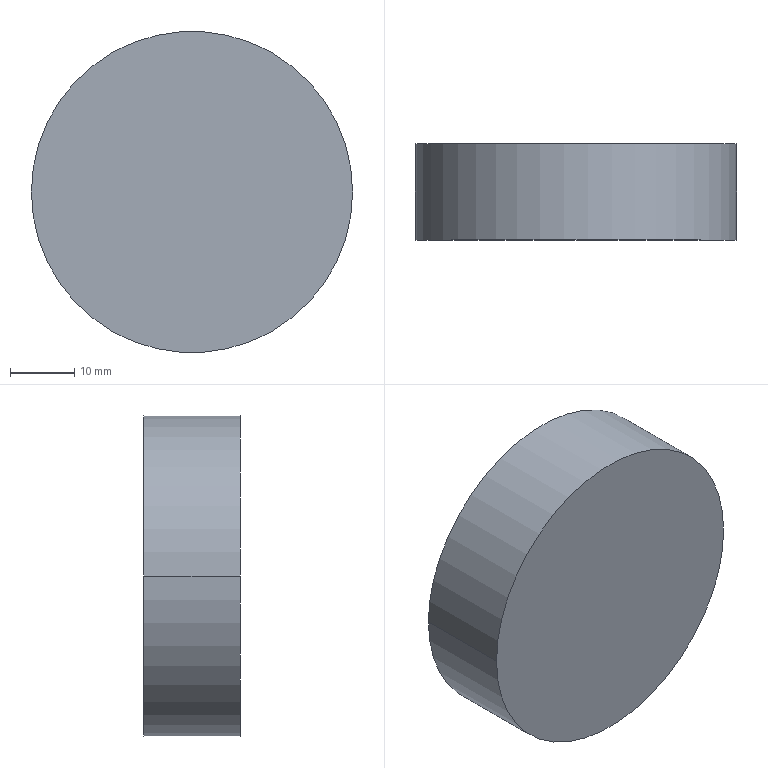Part | NX | 1 solid | 7 faces | box 50 x 15 x 50 mm | volume 11206 mm3 | cylinder 4 | plane 3 | commonest cylinder face diameters 44 x2 50 x2
STEP:
#1=CARTESIAN_POINT('',(-25.,0.,0.));
#2=VERTEX_POINT('',#1);
#3=CARTESIAN_POINT('',(25.,0.,0.));
#4=VERTEX_POINT('',#3);
#5=CARTESIAN_POINT('',(0.,0.,0.));
#6=DIRECTION('',(0.,1.,0.));
#7=DIRECTION('',(1.,0.,0.));
#8=AXIS2_PLACEMENT_3D('',#5,#6,#7);
#9=CIRCLE('',#8,25.);
#10=EDGE_CURVE('',#2,#4,#9,.T.);
#11=ORIENTED_EDGE('',*,*,#10,.F.);
#12=CARTESIAN_POINT('',(0.,0.,0.));
#13=DIRECTION('',(0.,1.,0.));
#14=DIRECTION('',(1.,0.,0.));
#15=AXIS2_PLACEMENT_3D('',#12,#13,#14);
#16=CIRCLE('',#15,25.);
#17=EDGE_CURVE('',#4,#2,#16,.T.);
#18=ORIENTED_EDGE('',*,*,#17,.F.);
#19=EDGE_LOOP('',(#11,#18));
#20=FACE_BOUND('',#19,.T.);
#21=CARTESIAN_POINT('',(0.,0.,0.));
#22=DIRECTION('',(0.,1.,0.));
#23=DIRECTION('',(1.,0.,0.));
#24=AXIS2_PLACEMENT_3D('',#21,#22,#23);
#25=PLANE('',#24);
#26=ADVANCED_FACE('',(#20),#25,.F.);
#27=ORIENTED_EDGE('',*,*,#10,.T.);
#28=CARTESIAN_POINT('',(25.,15.,0.));
#29=VERTEX_POINT('',#28);
#30=CARTESIAN_POINT('',(25.,0.,0.));
#31=DIRECTION('',(0.,1.,0.));
#32=VECTOR('',#31,1000.);
#33=LINE('',#30,#32);
#34=EDGE_CURVE('',#29,#4,#33,.F.);
#35=ORIENTED_EDGE('',*,*,#34,.F.);
#36=CARTESIAN_POINT('',(-25.,15.,0.));
#37=VERTEX_POINT('',#36);
#38=CARTESIAN_POINT('',(0.,15.,0.));
#39=DIRECTION('',(0.,-1.,0.));
#40=DIRECTION('',(-1.,0.,0.));
#41=AXIS2_PLACEMENT_3D('',#38,#39,#40);
#42=CIRCLE('',#41,25.);
#43=EDGE_CURVE('',#29,#37,#42,.T.);
#44=ORIENTED_EDGE('',*,*,#43,.T.);
#45=CARTESIAN_POINT('',(-25.,0.,0.));
#46=DIRECTION('',(0.,1.,0.));
#47=VECTOR('',#46,1000.);
#48=LINE('',#45,#47);
#49=EDGE_CURVE('',#37,#2,#48,.F.);
#50=ORIENTED_EDGE('',*,*,#49,.T.);
#51=EDGE_LOOP('',(#27,#35,#44,#50));
#52=FACE_BOUND('',#51,.T.);
#53=CARTESIAN_POINT('',(0.,0.,0.));
#54=DIRECTION('',(0.,1.,0.));
#55=DIRECTION('',(-1.,0.,0.));
#56=AXIS2_PLACEMENT_3D('',#53,#54,#55);
#57=CYLINDRICAL_SURFACE('',#56,25.);
#58=ADVANCED_FACE('',(#52),#57,.T.);
#59=CARTESIAN_POINT('',(-22.,3.,0.));
#60=VERTEX_POINT('',#59);
#61=CARTESIAN_POINT('',(22.,3.,0.));
#62=VERTEX_POINT('',#61);
#63=CARTESIAN_POINT('',(0.,3.,0.));
#64=DIRECTION('',(0.,-1.,0.));
#65=DIRECTION('',(1.,0.,0.));
#66=AXIS2_PLACEMENT_3D('',#63,#64,#65);
#67=CIRCLE('',#66,22.);
#68=EDGE_CURVE('',#60,#62,#67,.T.);
#69=ORIENTED_EDGE('',*,*,#68,.F.);
#70=CARTESIAN_POINT('',(0.,3.,0.));
#71=DIRECTION('',(0.,-1.,0.));
#72=DIRECTION('',(1.,0.,0.));
#73=AXIS2_PLACEMENT_3D('',#70,#71,#72);
#74=CIRCLE('',#73,22.);
#75=EDGE_CURVE('',#62,#60,#74,.T.);
#76=ORIENTED_EDGE('',*,*,#75,.F.);
#77=EDGE_LOOP('',(#69,#76));
#78=FACE_BOUND('',#77,.T.);
#79=CARTESIAN_POINT('',(0.,3.,0.));
#80=DIRECTION('',(0.,1.,0.));
#81=DIRECTION('',(1.,0.,0.));
#82=AXIS2_PLACEMENT_3D('',#79,#80,#81);
#83=PLANE('',#82);
#84=ADVANCED_FACE('',(#78),#83,.T.);
#85=ORIENTED_EDGE('',*,*,#43,.F.);
#86=CARTESIAN_POINT('',(0.,15.,0.));
#87=DIRECTION('',(0.,-1.,0.));
#88=DIRECTION('',(-1.,0.,0.));
#89=AXIS2_PLACEMENT_3D('',#86,#87,#88);
#90=CIRCLE('',#89,25.);
#91=EDGE_CURVE('',#37,#29,#90,.T.);
#92=ORIENTED_EDGE('',*,*,#91,.F.);
#93=EDGE_LOOP('',(#85,#92));
#94=FACE_BOUND('',#93,.T.);
#95=CARTESIAN_POINT('',(22.,15.,0.));
#96=VERTEX_POINT('',#95);
#97=CARTESIAN_POINT('',(-22.,15.,0.));
#98=VERTEX_POINT('',#97);
#99=CARTESIAN_POINT('',(0.,15.,0.));
#100=DIRECTION('',(0.,1.,0.));
#101=DIRECTION('',(1.,0.,0.));
#102=AXIS2_PLACEMENT_3D('',#99,#100,#101);
#103=CIRCLE('',#102,22.);
#104=EDGE_CURVE('',#96,#98,#103,.T.);
#105=ORIENTED_EDGE('',*,*,#104,.F.);
#106=CARTESIAN_POINT('',(0.,15.,0.));
#107=DIRECTION('',(0.,1.,0.));
#108=DIRECTION('',(1.,0.,0.));
#109=AXIS2_PLACEMENT_3D('',#106,#107,#108);
#110=CIRCLE('',#109,22.);
#111=EDGE_CURVE('',#98,#96,#110,.T.);
#112=ORIENTED_EDGE('',*,*,#111,.F.);
#113=EDGE_LOOP('',(#105,#112));
#114=FACE_BOUND('',#113,.T.);
#115=CARTESIAN_POINT('',(0.,15.,0.));
#116=DIRECTION('',(0.,1.,0.));
#117=DIRECTION('',(1.,0.,0.));
#118=AXIS2_PLACEMENT_3D('',#115,#116,#117);
#119=PLANE('',#118);
#120=ADVANCED_FACE('',(#94,#114),#119,.T.);
#121=ORIENTED_EDGE('',*,*,#104,.T.);
#122=CARTESIAN_POINT('',(-22.,0.,0.));
#123=DIRECTION('',(0.,1.,0.));
#124=VECTOR('',#123,1000.);
#125=LINE('',#122,#124);
#126=EDGE_CURVE('',#98,#60,#125,.F.);
#127=ORIENTED_EDGE('',*,*,#126,.T.);
#128=ORIENTED_EDGE('',*,*,#68,.T.);
#129=CARTESIAN_POINT('',(22.,0.,0.));
#130=DIRECTION('',(0.,1.,0.));
#131=VECTOR('',#130,1000.);
#132=LINE('',#129,#131);
#133=EDGE_CURVE('',#96,#62,#132,.F.);
#134=ORIENTED_EDGE('',*,*,#133,.F.);
#135=EDGE_LOOP('',(#121,#127,#128,#134));
#136=FACE_BOUND('',#135,.T.);
#137=CARTESIAN_POINT('',(0.,0.,0.));
#138=DIRECTION('',(0.,1.,0.));
#139=DIRECTION('',(-1.,0.,0.));
#140=AXIS2_PLACEMENT_3D('',#137,#138,#139);
#141=CYLINDRICAL_SURFACE('',#140,22.);
#142=ADVANCED_FACE('',(#136),#141,.F.);
#143=ORIENTED_EDGE('',*,*,#49,.F.);
#144=ORIENTED_EDGE('',*,*,#91,.T.);
#145=ORIENTED_EDGE('',*,*,#34,.T.);
#146=ORIENTED_EDGE('',*,*,#17,.T.);
#147=EDGE_LOOP('',(#143,#144,#145,#146));
#148=FACE_BOUND('',#147,.T.);
#149=CARTESIAN_POINT('',(0.,0.,0.));
#150=DIRECTION('',(0.,1.,0.));
#151=DIRECTION('',(-1.,0.,0.));
#152=AXIS2_PLACEMENT_3D('',#149,#150,#151);
#153=CYLINDRICAL_SURFACE('',#152,25.);
#154=ADVANCED_FACE('',(#148),#153,.T.);
#155=ORIENTED_EDGE('',*,*,#126,.F.);
#156=ORIENTED_EDGE('',*,*,#111,.T.);
#157=ORIENTED_EDGE('',*,*,#133,.T.);
#158=ORIENTED_EDGE('',*,*,#75,.T.);
#159=EDGE_LOOP('',(#155,#156,#157,#158));
#160=FACE_BOUND('',#159,.T.);
#161=CARTESIAN_POINT('',(0.,0.,0.));
#162=DIRECTION('',(0.,1.,0.));
#163=DIRECTION('',(-1.,0.,0.));
#164=AXIS2_PLACEMENT_3D('',#161,#162,#163);
#165=CYLINDRICAL_SURFACE('',#164,22.);
#166=ADVANCED_FACE('',(#160),#165,.F.);
#167=CLOSED_SHELL('',(#26,#58,#84,#120,#142,#154,#166));
#168=MANIFOLD_SOLID_BREP('',#167);
#169=(LENGTH_UNIT()NAMED_UNIT(*)SI_UNIT(.MILLI.,.METRE.));
#170=UNCERTAINTY_MEASURE_WITH_UNIT(LENGTH_MEASURE(0.00001),#169,'','');
#171=(NAMED_UNIT(*)PLANE_ANGLE_UNIT()SI_UNIT($,.RADIAN.));
#172=(NAMED_UNIT(*)SI_UNIT($,.STERADIAN.)SOLID_ANGLE_UNIT());
#173=(GEOMETRIC_REPRESENTATION_CONTEXT(3)GLOBAL_UNCERTAINTY_ASSIGNED_CONTEXT((#170))GLOBAL_UNIT_ASSIGNED_CONTEXT((#169,#171,#172))REPRESENTATION_CONTEXT('',''));
#174=ADVANCED_BREP_SHAPE_REPRESENTATION('',(#168),#173);